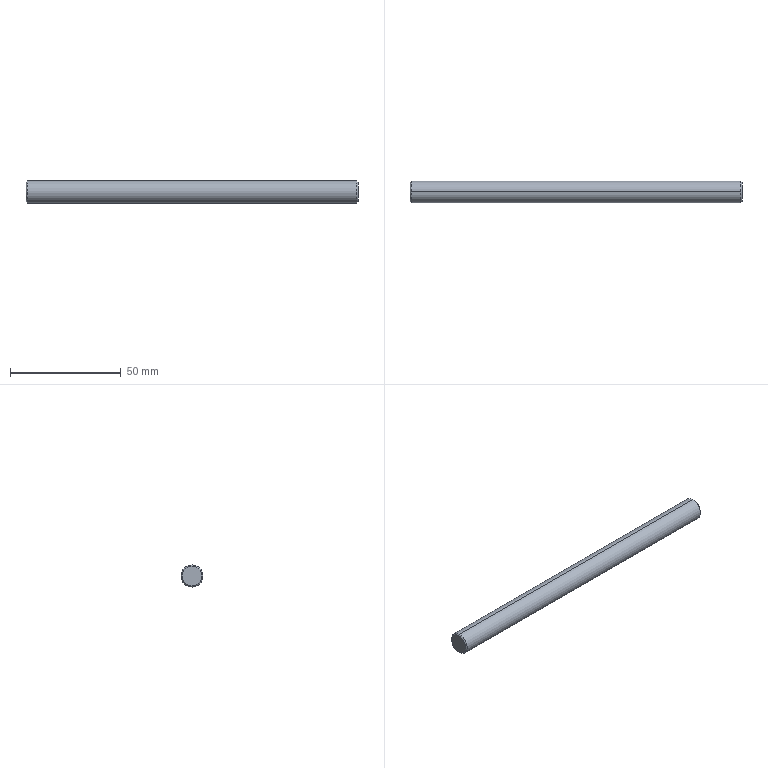Part | STEP file | 03-18 Φ10 suction mechanism guide post | 1 solid | 14 faces | box 150 x 10 x 10 mm | volume 11525 mm3 | cone 8 | cylinder 4 | plane 2 | commonest cylinder face diameters 4.2 x2 10 x2